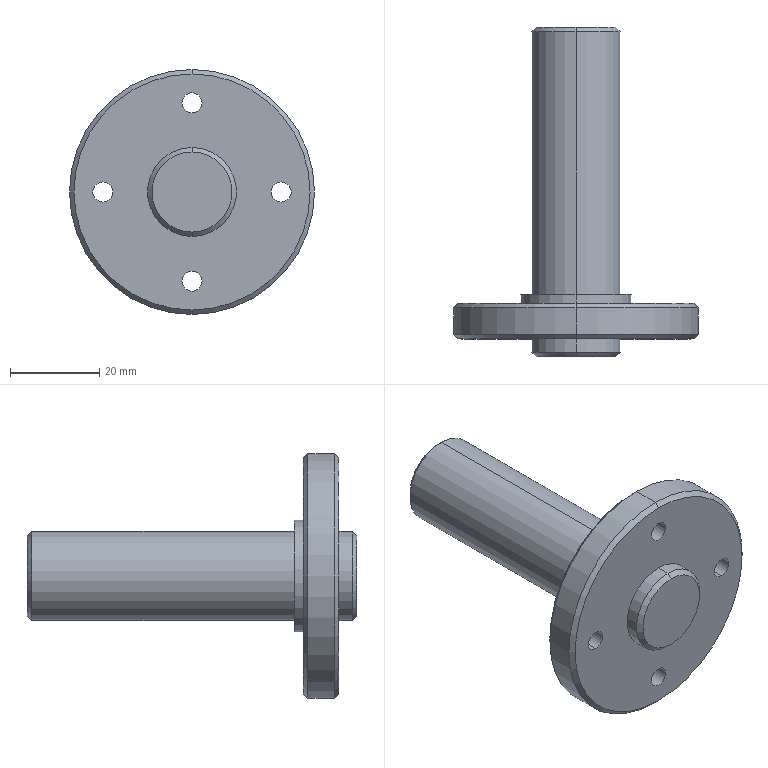Part | NX | features 00 2 | 1 solid | 41 faces | box 55 x 74 x 55 mm | volume 38722 mm3 | cylinder 24 | plane 9 | cone 8 | commonest cylinder face diameters 4.5 x8 8 x8 20 x4 25 x2 55 x2
STEP:
#1=CARTESIAN_POINT('',(0.,119.,-258.129));
#2=VERTEX_POINT('',#1);
#3=CARTESIAN_POINT('',(0.,119.,-278.129));
#4=VERTEX_POINT('',#3);
#5=CARTESIAN_POINT('',(0.,119.,-268.129));
#6=DIRECTION('',(0.,1.,0.));
#7=DIRECTION('',(0.,0.,1.));
#8=AXIS2_PLACEMENT_3D('',#5,#6,#7);
#9=CIRCLE('',#8,10.);
#10=EDGE_CURVE('',#2,#4,#9,.T.);
#11=ORIENTED_EDGE('',*,*,#10,.F.);
#12=CARTESIAN_POINT('',(0.,60.,-258.129));
#13=VERTEX_POINT('',#12);
#14=CARTESIAN_POINT('',(0.,60.,-258.129));
#15=DIRECTION('',(0.,1.,0.));
#16=VECTOR('',#15,1000.);
#17=LINE('',#14,#16);
#18=EDGE_CURVE('',#13,#2,#17,.T.);
#19=ORIENTED_EDGE('',*,*,#18,.F.);
#20=CARTESIAN_POINT('',(0.,60.,-278.129));
#21=VERTEX_POINT('',#20);
#22=CARTESIAN_POINT('',(0.,60.,-268.129));
#23=DIRECTION('',(0.,-1.,0.));
#24=DIRECTION('',(0.,0.,-1.));
#25=AXIS2_PLACEMENT_3D('',#22,#23,#24);
#26=CIRCLE('',#25,10.);
#27=EDGE_CURVE('',#21,#13,#26,.T.);
#28=ORIENTED_EDGE('',*,*,#27,.F.);
#29=CARTESIAN_POINT('',(0.,60.,-278.129));
#30=DIRECTION('',(0.,1.,0.));
#31=VECTOR('',#30,1000.);
#32=LINE('',#29,#31);
#33=EDGE_CURVE('',#4,#21,#32,.F.);
#34=ORIENTED_EDGE('',*,*,#33,.F.);
#35=EDGE_LOOP('',(#11,#19,#28,#34));
#36=FACE_BOUND('',#35,.T.);
#37=CARTESIAN_POINT('',(0.,50.,-268.129));
#38=DIRECTION('',(0.,-1.,0.));
#39=DIRECTION('',(0.,0.,1.));
#40=AXIS2_PLACEMENT_3D('',#37,#38,#39);
#41=CYLINDRICAL_SURFACE('',#40,10.);
#42=ADVANCED_FACE('',(#36),#41,.T.);
#43=CARTESIAN_POINT('',(0.,120.,-259.129));
#44=VERTEX_POINT('',#43);
#45=CARTESIAN_POINT('',(0.,120.,-277.129));
#46=VERTEX_POINT('',#45);
#47=CARTESIAN_POINT('',(0.,120.,-268.129));
#48=DIRECTION('',(0.,1.,0.));
#49=DIRECTION('',(0.,0.,1.));
#50=AXIS2_PLACEMENT_3D('',#47,#48,#49);
#51=CIRCLE('',#50,9.);
#52=EDGE_CURVE('',#44,#46,#51,.T.);
#53=ORIENTED_EDGE('',*,*,#52,.F.);
#54=CARTESIAN_POINT('',(0.,119.,-258.129));
#55=DIRECTION('',(0.,0.7071,-0.7071));
#56=VECTOR('',#55,1000.);
#57=LINE('',#54,#56);
#58=EDGE_CURVE('',#44,#2,#57,.F.);
#59=ORIENTED_EDGE('',*,*,#58,.T.);
#60=ORIENTED_EDGE('',*,*,#10,.T.);
#61=CARTESIAN_POINT('',(0.,119.,-278.129));
#62=DIRECTION('',(0.,0.7071,0.7071));
#63=VECTOR('',#62,1000.);
#64=LINE('',#61,#63);
#65=EDGE_CURVE('',#4,#46,#64,.T.);
#66=ORIENTED_EDGE('',*,*,#65,.T.);
#67=EDGE_LOOP('',(#53,#59,#60,#66));
#68=FACE_BOUND('',#67,.T.);
#69=CARTESIAN_POINT('',(0.,120.091,-268.129));
#70=DIRECTION('',(0.,-1.,0.));
#71=DIRECTION('',(0.,0.,1.));
#72=AXIS2_PLACEMENT_3D('',#69,#70,#71);
#73=CONICAL_SURFACE('',#72,8.909,0.7854);
#74=ADVANCED_FACE('',(#68),#73,.T.);
#75=CARTESIAN_POINT('',(0.,120.,-268.129));
#76=DIRECTION('',(0.,1.,0.));
#77=DIRECTION('',(0.,0.,-1.));
#78=AXIS2_PLACEMENT_3D('',#75,#76,#77);
#79=CIRCLE('',#78,9.);
#80=EDGE_CURVE('',#46,#44,#79,.T.);
#81=ORIENTED_EDGE('',*,*,#80,.T.);
#82=ORIENTED_EDGE('',*,*,#52,.T.);
#83=EDGE_LOOP('',(#81,#82));
#84=FACE_BOUND('',#83,.T.);
#85=CARTESIAN_POINT('',(-10.,120.,-268.129));
#86=DIRECTION('',(0.,1.,0.));
#87=DIRECTION('',(0.,0.,-1.));
#88=AXIS2_PLACEMENT_3D('',#85,#86,#87);
#89=PLANE('',#88);
#90=ADVANCED_FACE('',(#84),#89,.T.);
#91=ORIENTED_EDGE('',*,*,#65,.F.);
#92=CARTESIAN_POINT('',(0.,119.,-268.129));
#93=DIRECTION('',(0.,1.,0.));
#94=DIRECTION('',(0.,0.,-1.));
#95=AXIS2_PLACEMENT_3D('',#92,#93,#94);
#96=CIRCLE('',#95,10.);
#97=EDGE_CURVE('',#4,#2,#96,.T.);
#98=ORIENTED_EDGE('',*,*,#97,.T.);
#99=ORIENTED_EDGE('',*,*,#58,.F.);
#100=ORIENTED_EDGE('',*,*,#80,.F.);
#101=EDGE_LOOP('',(#91,#98,#99,#100));
#102=FACE_BOUND('',#101,.T.);
#103=CARTESIAN_POINT('',(0.,120.091,-268.129));
#104=DIRECTION('',(0.,-1.,0.));
#105=DIRECTION('',(0.,0.,1.));
#106=AXIS2_PLACEMENT_3D('',#103,#104,#105);
#107=CONICAL_SURFACE('',#106,8.909,0.7854);
#108=ADVANCED_FACE('',(#102),#107,.T.);
#109=ORIENTED_EDGE('',*,*,#33,.T.);
#110=CARTESIAN_POINT('',(0.,60.,-268.129));
#111=DIRECTION('',(0.,-1.,0.));
#112=DIRECTION('',(0.,0.,1.));
#113=AXIS2_PLACEMENT_3D('',#110,#111,#112);
#114=CIRCLE('',#113,10.);
#115=EDGE_CURVE('',#13,#21,#114,.T.);
#116=ORIENTED_EDGE('',*,*,#115,.F.);
#117=ORIENTED_EDGE('',*,*,#18,.T.);
#118=ORIENTED_EDGE('',*,*,#97,.F.);
#119=EDGE_LOOP('',(#109,#116,#117,#118));
#120=FACE_BOUND('',#119,.T.);
#121=CARTESIAN_POINT('',(0.,50.,-268.129));
#122=DIRECTION('',(0.,-1.,0.));
#123=DIRECTION('',(0.,0.,1.));
#124=AXIS2_PLACEMENT_3D('',#121,#122,#123);
#125=CYLINDRICAL_SURFACE('',#124,10.);
#126=ADVANCED_FACE('',(#120),#125,.T.);
#127=CARTESIAN_POINT('',(0.,60.,-255.629));
#128=VERTEX_POINT('',#127);
#129=CARTESIAN_POINT('',(0.,60.,-280.629));
#130=VERTEX_POINT('',#129);
#131=CARTESIAN_POINT('',(0.,60.,-268.129));
#132=DIRECTION('',(0.,1.,0.));
#133=DIRECTION('',(0.,0.,1.));
#134=AXIS2_PLACEMENT_3D('',#131,#132,#133);
#135=CIRCLE('',#134,12.5);
#136=EDGE_CURVE('',#128,#130,#135,.T.);
#137=ORIENTED_EDGE('',*,*,#136,.F.);
#138=CARTESIAN_POINT('',(0.,58.,-255.629));
#139=VERTEX_POINT('',#138);
#140=CARTESIAN_POINT('',(0.,58.,-255.629));
#141=DIRECTION('',(0.,1.,0.));
#142=VECTOR('',#141,1000.);
#143=LINE('',#140,#142);
#144=EDGE_CURVE('',#128,#139,#143,.F.);
#145=ORIENTED_EDGE('',*,*,#144,.T.);
#146=CARTESIAN_POINT('',(0.,58.,-280.629));
#147=VERTEX_POINT('',#146);
#148=CARTESIAN_POINT('',(0.,58.,-268.129));
#149=DIRECTION('',(0.,-1.,0.));
#150=DIRECTION('',(0.,0.,-1.));
#151=AXIS2_PLACEMENT_3D('',#148,#149,#150);
#152=CIRCLE('',#151,12.5);
#153=EDGE_CURVE('',#147,#139,#152,.T.);
#154=ORIENTED_EDGE('',*,*,#153,.F.);
#155=CARTESIAN_POINT('',(0.,58.,-280.629));
#156=DIRECTION('',(0.,1.,0.));
#157=VECTOR('',#156,1000.);
#158=LINE('',#155,#157);
#159=EDGE_CURVE('',#147,#130,#158,.T.);
#160=ORIENTED_EDGE('',*,*,#159,.T.);
#161=EDGE_LOOP('',(#137,#145,#154,#160));
#162=FACE_BOUND('',#161,.T.);
#163=CARTESIAN_POINT('',(0.,50.,-268.129));
#164=DIRECTION('',(0.,-1.,0.));
#165=DIRECTION('',(0.,0.,1.));
#166=AXIS2_PLACEMENT_3D('',#163,#164,#165);
#167=CYLINDRICAL_SURFACE('',#166,12.5);
#168=ADVANCED_FACE('',(#162),#167,.T.);
#169=ORIENTED_EDGE('',*,*,#27,.T.);
#170=ORIENTED_EDGE('',*,*,#115,.T.);
#171=EDGE_LOOP('',(#169,#170));
#172=FACE_BOUND('',#171,.T.);
#173=ORIENTED_EDGE('',*,*,#136,.T.);
#174=CARTESIAN_POINT('',(0.,60.,-268.129));
#175=DIRECTION('',(0.,1.,0.));
#176=DIRECTION('',(0.,0.,-1.));
#177=AXIS2_PLACEMENT_3D('',#174,#175,#176);
#178=CIRCLE('',#177,12.5);
#179=EDGE_CURVE('',#130,#128,#178,.T.);
#180=ORIENTED_EDGE('',*,*,#179,.T.);
#181=EDGE_LOOP('',(#173,#180));
#182=FACE_BOUND('',#181,.T.);
#183=CARTESIAN_POINT('',(-12.5,60.,-268.129));
#184=DIRECTION('',(0.,1.,0.));
#185=DIRECTION('',(0.,0.,-1.));
#186=AXIS2_PLACEMENT_3D('',#183,#184,#185);
#187=PLANE('',#186);
#188=ADVANCED_FACE('',(#172,#182),#187,.T.);
#189=ORIENTED_EDGE('',*,*,#159,.F.);
#190=CARTESIAN_POINT('',(0.,58.,-268.129));
#191=DIRECTION('',(0.,-1.,0.));
#192=DIRECTION('',(0.,0.,1.));
#193=AXIS2_PLACEMENT_3D('',#190,#191,#192);
#194=CIRCLE('',#193,12.5);
#195=EDGE_CURVE('',#139,#147,#194,.T.);
#196=ORIENTED_EDGE('',*,*,#195,.F.);
#197=ORIENTED_EDGE('',*,*,#144,.F.);
#198=ORIENTED_EDGE('',*,*,#179,.F.);
#199=EDGE_LOOP('',(#189,#196,#197,#198));
#200=FACE_BOUND('',#199,.T.);
#201=CARTESIAN_POINT('',(0.,50.,-268.129));
#202=DIRECTION('',(0.,-1.,0.));
#203=DIRECTION('',(0.,0.,1.));
#204=AXIS2_PLACEMENT_3D('',#201,#202,#203);
#205=CYLINDRICAL_SURFACE('',#204,12.5);
#206=ADVANCED_FACE('',(#200),#205,.T.);
#207=CARTESIAN_POINT('',(-20.,53.4,-265.879));
#208=VERTEX_POINT('',#207);
#209=CARTESIAN_POINT('',(-20.,50.,-265.879));
#210=VERTEX_POINT('',#209);
#211=CARTESIAN_POINT('',(-20.,53.4,-265.879));
#212=DIRECTION('',(0.,-1.,0.));
#213=VECTOR('',#212,1000.);
#214=LINE('',#211,#213);
#215=EDGE_CURVE('',#208,#210,#214,.T.);
#216=ORIENTED_EDGE('',*,*,#215,.F.);
#217=CARTESIAN_POINT('',(-20.,53.4,-270.379));
#218=VERTEX_POINT('',#217);
#219=CARTESIAN_POINT('',(-20.,53.4,-268.129));
#220=DIRECTION('',(0.,-1.,0.));
#221=DIRECTION('',(0.,0.,-1.));
#222=AXIS2_PLACEMENT_3D('',#219,#220,#221);
#223=CIRCLE('',#222,2.25);
#224=EDGE_CURVE('',#218,#208,#223,.T.);
#225=ORIENTED_EDGE('',*,*,#224,.F.);
#226=CARTESIAN_POINT('',(-20.,50.,-270.379));
#227=VERTEX_POINT('',#226);
#228=CARTESIAN_POINT('',(-20.,53.4,-270.379));
#229=DIRECTION('',(0.,-1.,0.));
#230=VECTOR('',#229,1000.);
#231=LINE('',#228,#230);
#232=EDGE_CURVE('',#227,#218,#231,.F.);
#233=ORIENTED_EDGE('',*,*,#232,.F.);
#234=CARTESIAN_POINT('',(-20.,50.,-268.129));
#235=DIRECTION('',(0.,1.,0.));
#236=DIRECTION('',(0.,0.,1.));
#237=AXIS2_PLACEMENT_3D('',#234,#235,#236);
#238=CIRCLE('',#237,2.25);
#239=EDGE_CURVE('',#210,#227,#238,.T.);
#240=ORIENTED_EDGE('',*,*,#239,.F.);
#241=EDGE_LOOP('',(#216,#225,#233,#240));
#242=FACE_BOUND('',#241,.T.);
#243=CARTESIAN_POINT('',(-20.,58.,-268.129));
#244=DIRECTION('',(0.,1.,0.));
#245=DIRECTION('',(0.,0.,-1.));
#246=AXIS2_PLACEMENT_3D('',#243,#244,#245);
#247=CYLINDRICAL_SURFACE('',#246,2.25);
#248=ADVANCED_FACE('',(#242),#247,.F.);
#249=CARTESIAN_POINT('',(-20.,50.,-268.129));
#250=DIRECTION('',(0.,1.,0.));
#251=DIRECTION('',(0.,0.,-1.));
#252=AXIS2_PLACEMENT_3D('',#249,#250,#251);
#253=CIRCLE('',#252,2.25);
#254=EDGE_CURVE('',#227,#210,#253,.T.);
#255=ORIENTED_EDGE('',*,*,#254,.F.);
#256=ORIENTED_EDGE('',*,*,#232,.T.);
#257=CARTESIAN_POINT('',(-20.,53.4,-268.129));
#258=DIRECTION('',(0.,-1.,0.));
#259=DIRECTION('',(0.,0.,1.));
#260=AXIS2_PLACEMENT_3D('',#257,#258,#259);
#261=CIRCLE('',#260,2.25);
#262=EDGE_CURVE('',#208,#218,#261,.T.);
#263=ORIENTED_EDGE('',*,*,#262,.F.);
#264=ORIENTED_EDGE('',*,*,#215,.T.);
#265=EDGE_LOOP('',(#255,#256,#263,#264));
#266=FACE_BOUND('',#265,.T.);
#267=CARTESIAN_POINT('',(-20.,58.,-268.129));
#268=DIRECTION('',(0.,1.,0.));
#269=DIRECTION('',(0.,0.,-1.));
#270=AXIS2_PLACEMENT_3D('',#267,#268,#269);
#271=CYLINDRICAL_SURFACE('',#270,2.25);
#272=ADVANCED_FACE('',(#266),#271,.F.);
#273=ORIENTED_EDGE('',*,*,#224,.T.);
#274=ORIENTED_EDGE('',*,*,#262,.T.);
#275=EDGE_LOOP('',(#273,#274));
#276=FACE_BOUND('',#275,.T.);
#277=CARTESIAN_POINT('',(-20.,53.4,-264.129));
#278=VERTEX_POINT('',#277);
#279=CARTESIAN_POINT('',(-20.,53.4,-272.129));
#280=VERTEX_POINT('',#279);
#281=CARTESIAN_POINT('',(-20.,53.4,-268.129));
#282=DIRECTION('',(0.,1.,0.));
#283=DIRECTION('',(0.,0.,1.));
#284=AXIS2_PLACEMENT_3D('',#281,#282,#283);
#285=CIRCLE('',#284,4.);
#286=EDGE_CURVE('',#278,#280,#285,.T.);
#287=ORIENTED_EDGE('',*,*,#286,.T.);
#288=CARTESIAN_POINT('',(-20.,53.4,-268.129));
#289=DIRECTION('',(0.,1.,0.));
#290=DIRECTION('',(0.,0.,-1.));
#291=AXIS2_PLACEMENT_3D('',#288,#289,#290);
#292=CIRCLE('',#291,4.);
#293=EDGE_CURVE('',#280,#278,#292,.T.);
#294=ORIENTED_EDGE('',*,*,#293,.T.);
#295=EDGE_LOOP('',(#287,#294));
#296=FACE_BOUND('',#295,.T.);
#297=CARTESIAN_POINT('',(-22.25,53.4,-268.129));
#298=DIRECTION('',(0.,-1.,0.));
#299=DIRECTION('',(0.,0.,1.));
#300=AXIS2_PLACEMENT_3D('',#297,#298,#299);
#301=PLANE('',#300);
#302=ADVANCED_FACE('',(#276,#296),#301,.F.);
#303=CARTESIAN_POINT('',(-20.,58.,-264.129));
#304=VERTEX_POINT('',#303);
#305=CARTESIAN_POINT('',(-20.,58.,-264.129));
#306=DIRECTION('',(0.,-1.,0.));
#307=VECTOR('',#306,1000.);
#308=LINE('',#305,#307);
#309=EDGE_CURVE('',#304,#278,#308,.T.);
#310=ORIENTED_EDGE('',*,*,#309,.F.);
#311=CARTESIAN_POINT('',(-20.,58.,-272.129));
#312=VERTEX_POINT('',#311);
#313=CARTESIAN_POINT('',(-20.,58.,-268.129));
#314=DIRECTION('',(0.,-1.,0.));
#315=DIRECTION('',(0.,0.,-1.));
#316=AXIS2_PLACEMENT_3D('',#313,#314,#315);
#317=CIRCLE('',#316,4.);
#318=EDGE_CURVE('',#312,#304,#317,.T.);
#319=ORIENTED_EDGE('',*,*,#318,.F.);
#320=CARTESIAN_POINT('',(-20.,58.,-272.129));
#321=DIRECTION('',(0.,-1.,0.));
#322=VECTOR('',#321,1000.);
#323=LINE('',#320,#322);
#324=EDGE_CURVE('',#280,#312,#323,.F.);
#325=ORIENTED_EDGE('',*,*,#324,.F.);
#326=ORIENTED_EDGE('',*,*,#286,.F.);
#327=EDGE_LOOP('',(#310,#319,#325,#326));
#328=FACE_BOUND('',#327,.T.);
#329=CARTESIAN_POINT('',(-20.,58.,-268.129));
#330=DIRECTION('',(0.,1.,0.));
#331=DIRECTION('',(0.,0.,-1.));
#332=AXIS2_PLACEMENT_3D('',#329,#330,#331);
#333=CYLINDRICAL_SURFACE('',#332,4.);
#334=ADVANCED_FACE('',(#328),#333,.F.);
#335=ORIENTED_EDGE('',*,*,#293,.F.);
#336=ORIENTED_EDGE('',*,*,#324,.T.);
#337=CARTESIAN_POINT('',(-20.,58.,-268.129));
#338=DIRECTION('',(0.,-1.,0.));
#339=DIRECTION('',(0.,0.,1.));
#340=AXIS2_PLACEMENT_3D('',#337,#338,#339);
#341=CIRCLE('',#340,4.);
#342=EDGE_CURVE('',#304,#312,#341,.T.);
#343=ORIENTED_EDGE('',*,*,#342,.F.);
#344=ORIENTED_EDGE('',*,*,#309,.T.);
#345=EDGE_LOOP('',(#335,#336,#343,#344));
#346=FACE_BOUND('',#345,.T.);
#347=CARTESIAN_POINT('',(-20.,58.,-268.129));
#348=DIRECTION('',(0.,1.,0.));
#349=DIRECTION('',(0.,0.,-1.));
#350=AXIS2_PLACEMENT_3D('',#347,#348,#349);
#351=CYLINDRICAL_SURFACE('',#350,4.);
#352=ADVANCED_FACE('',(#346),#351,.F.);
#353=CARTESIAN_POINT('',(-2.25,50.,-288.129));
#354=VERTEX_POINT('',#353);
#355=CARTESIAN_POINT('',(-2.25,53.4,-288.129));
#356=VERTEX_POINT('',#355);
#357=CARTESIAN_POINT('',(-2.25,53.4,-288.129));
#358=DIRECTION('',(0.,-1.,0.));
#359=VECTOR('',#358,1000.);
#360=LINE('',#357,#359);
#361=EDGE_CURVE('',#354,#356,#360,.F.);
#362=ORIENTED_EDGE('',*,*,#361,.T.);
#363=CARTESIAN_POINT('',(2.25,53.4,-288.129));
#364=VERTEX_POINT('',#363);
#365=CARTESIAN_POINT('',(0.,53.4,-288.129));
#366=DIRECTION('',(0.,-1.,0.));
#367=DIRECTION('',(1.,0.,0.));
#368=AXIS2_PLACEMENT_3D('',#365,#366,#367);
#369=CIRCLE('',#368,2.25);
#370=EDGE_CURVE('',#364,#356,#369,.T.);
#371=ORIENTED_EDGE('',*,*,#370,.F.);
#372=CARTESIAN_POINT('',(2.25,50.,-288.129));
#373=VERTEX_POINT('',#372);
#374=CARTESIAN_POINT('',(2.25,53.4,-288.129));
#375=DIRECTION('',(0.,-1.,0.));
#376=VECTOR('',#375,1000.);
#377=LINE('',#374,#376);
#378=EDGE_CURVE('',#364,#373,#377,.T.);
#379=ORIENTED_EDGE('',*,*,#378,.T.);
#380=CARTESIAN_POINT('',(0.,50.,-288.129));
#381=DIRECTION('',(0.,1.,0.));
#382=DIRECTION('',(-1.,0.,0.));
#383=AXIS2_PLACEMENT_3D('',#380,#381,#382);
#384=CIRCLE('',#383,2.25);
#385=EDGE_CURVE('',#354,#373,#384,.T.);
#386=ORIENTED_EDGE('',*,*,#385,.F.);
#387=EDGE_LOOP('',(#362,#371,#379,#386));
#388=FACE_BOUND('',#387,.T.);
#389=CARTESIAN_POINT('',(0.,58.,-288.129));
#390=DIRECTION('',(0.,1.,0.));
#391=DIRECTION('',(1.,0.,0.));
#392=AXIS2_PLACEMENT_3D('',#389,#390,#391);
#393=CYLINDRICAL_SURFACE('',#392,2.25);
#394=ADVANCED_FACE('',(#388),#393,.F.);
#395=CARTESIAN_POINT('',(0.,50.,-288.129));
#396=DIRECTION('',(0.,1.,0.));
#397=DIRECTION('',(1.,0.,0.));
#398=AXIS2_PLACEMENT_3D('',#395,#396,#397);
#399=CIRCLE('',#398,2.25);
#400=EDGE_CURVE('',#373,#354,#399,.T.);
#401=ORIENTED_EDGE('',*,*,#400,.F.);
#402=ORIENTED_EDGE('',*,*,#378,.F.);
#403=CARTESIAN_POINT('',(0.,53.4,-288.129));
#404=DIRECTION('',(0.,-1.,0.));
#405=DIRECTION('',(-1.,0.,0.));
#406=AXIS2_PLACEMENT_3D('',#403,#404,#405);
#407=CIRCLE('',#406,2.25);
#408=EDGE_CURVE('',#356,#364,#407,.T.);
#409=ORIENTED_EDGE('',*,*,#408,.F.);
#410=ORIENTED_EDGE('',*,*,#361,.F.);
#411=EDGE_LOOP('',(#401,#402,#409,#410));
#412=FACE_BOUND('',#411,.T.);
#413=CARTESIAN_POINT('',(0.,58.,-288.129));
#414=DIRECTION('',(0.,1.,0.));
#415=DIRECTION('',(1.,0.,0.));
#416=AXIS2_PLACEMENT_3D('',#413,#414,#415);
#417=CYLINDRICAL_SURFACE('',#416,2.25);
#418=ADVANCED_FACE('',(#412),#417,.F.);
#419=ORIENTED_EDGE('',*,*,#370,.T.);
#420=ORIENTED_EDGE('',*,*,#408,.T.);
#421=EDGE_LOOP('',(#419,#420));
#422=FACE_BOUND('',#421,.T.);
#423=CARTESIAN_POINT('',(-4.,53.4,-288.129));
#424=VERTEX_POINT('',#423);
#425=CARTESIAN_POINT('',(4.,53.4,-288.129));
#426=VERTEX_POINT('',#425);
#427=CARTESIAN_POINT('',(0.,53.4,-288.129));
#428=DIRECTION('',(0.,1.,0.));
#429=DIRECTION('',(-1.,0.,0.));
#430=AXIS2_PLACEMENT_3D('',#427,#428,#429);
#431=CIRCLE('',#430,4.);
#432=EDGE_CURVE('',#424,#426,#431,.T.);
#433=ORIENTED_EDGE('',*,*,#432,.T.);
#434=CARTESIAN_POINT('',(0.,53.4,-288.129));
#435=DIRECTION('',(0.,1.,0.));
#436=DIRECTION('',(1.,0.,0.));
#437=AXIS2_PLACEMENT_3D('',#434,#435,#436);
#438=CIRCLE('',#437,4.);
#439=EDGE_CURVE('',#426,#424,#438,.T.);
#440=ORIENTED_EDGE('',*,*,#439,.T.);
#441=EDGE_LOOP('',(#433,#440));
#442=FACE_BOUND('',#441,.T.);
#443=CARTESIAN_POINT('',(0.,53.4,-290.379));
#444=DIRECTION('',(0.,-1.,0.));
#445=DIRECTION('',(-1.,0.,0.));
#446=AXIS2_PLACEMENT_3D('',#443,#444,#445);
#447=PLANE('',#446);
#448=ADVANCED_FACE('',(#422,#442),#447,.F.);
#449=CARTESIAN_POINT('',(-4.,58.,-288.129));
#450=VERTEX_POINT('',#449);
#451=CARTESIAN_POINT('',(-4.,58.,-288.129));
#452=DIRECTION('',(0.,-1.,0.));
#453=VECTOR('',#452,1000.);
#454=LINE('',#451,#453);
#455=EDGE_CURVE('',#450,#424,#454,.T.);
#456=ORIENTED_EDGE('',*,*,#455,.F.);
#457=CARTESIAN_POINT('',(4.,58.,-288.129));
#458=VERTEX_POINT('',#457);
#459=CARTESIAN_POINT('',(0.,58.,-288.129));
#460=DIRECTION('',(0.,-1.,0.));
#461=DIRECTION('',(1.,0.,0.));
#462=AXIS2_PLACEMENT_3D('',#459,#460,#461);
#463=CIRCLE('',#462,4.);
#464=EDGE_CURVE('',#458,#450,#463,.T.);
#465=ORIENTED_EDGE('',*,*,#464,.F.);
#466=CARTESIAN_POINT('',(4.,58.,-288.129));
#467=DIRECTION('',(0.,-1.,0.));
#468=VECTOR('',#467,1000.);
#469=LINE('',#466,#468);
#470=EDGE_CURVE('',#426,#458,#469,.F.);
#471=ORIENTED_EDGE('',*,*,#470,.F.);
#472=ORIENTED_EDGE('',*,*,#432,.F.);
#473=EDGE_LOOP('',(#456,#465,#471,#472));
#474=FACE_BOUND('',#473,.T.);
#475=CARTESIAN_POINT('',(0.,58.,-288.129));
#476=DIRECTION('',(0.,1.,0.));
#477=DIRECTION('',(1.,0.,0.));
#478=AXIS2_PLACEMENT_3D('',#475,#476,#477);
#479=CYLINDRICAL_SURFACE('',#478,4.);
#480=ADVANCED_FACE('',(#474),#479,.F.);
#481=ORIENTED_EDGE('',*,*,#439,.F.);
#482=ORIENTED_EDGE('',*,*,#470,.T.);
#483=CARTESIAN_POINT('',(0.,58.,-288.129));
#484=DIRECTION('',(0.,-1.,0.));
#485=DIRECTION('',(-1.,0.,0.));
#486=AXIS2_PLACEMENT_3D('',#483,#484,#485);
#487=CIRCLE('',#486,4.);
#488=EDGE_CURVE('',#450,#458,#487,.T.);
#489=ORIENTED_EDGE('',*,*,#488,.F.);
#490=ORIENTED_EDGE('',*,*,#455,.T.);
#491=EDGE_LOOP('',(#481,#482,#489,#490));
#492=FACE_BOUND('',#491,.T.);
#493=CARTESIAN_POINT('',(0.,58.,-288.129));
#494=DIRECTION('',(0.,1.,0.));
#495=DIRECTION('',(1.,0.,0.));
#496=AXIS2_PLACEMENT_3D('',#493,#494,#495);
#497=CYLINDRICAL_SURFACE('',#496,4.);
#498=ADVANCED_FACE('',(#492),#497,.F.);
#499=CARTESIAN_POINT('',(20.,53.4,-270.379));
#500=VERTEX_POINT('',#499);
#501=CARTESIAN_POINT('',(20.,50.,-270.379));
#502=VERTEX_POINT('',#501);
#503=CARTESIAN_POINT('',(20.,53.4,-270.379));
#504=DIRECTION('',(0.,-1.,0.));
#505=VECTOR('',#504,1000.);
#506=LINE('',#503,#505);
#507=EDGE_CURVE('',#500,#502,#506,.T.);
#508=ORIENTED_EDGE('',*,*,#507,.F.);
#509=CARTESIAN_POINT('',(20.,53.4,-265.879));
#510=VERTEX_POINT('',#509);
#511=CARTESIAN_POINT('',(20.,53.4,-268.129));
#512=DIRECTION('',(0.,-1.,0.));
#513=DIRECTION('',(0.,0.,1.));
#514=AXIS2_PLACEMENT_3D('',#511,#512,#513);
#515=CIRCLE('',#514,2.25);
#516=EDGE_CURVE('',#510,#500,#515,.T.);
#517=ORIENTED_EDGE('',*,*,#516,.F.);
#518=CARTESIAN_POINT('',(20.,50.,-265.879));
#519=VERTEX_POINT('',#518);
#520=CARTESIAN_POINT('',(20.,53.4,-265.879));
#521=DIRECTION('',(0.,-1.,0.));
#522=VECTOR('',#521,1000.);
#523=LINE('',#520,#522);
#524=EDGE_CURVE('',#519,#510,#523,.F.);
#525=ORIENTED_EDGE('',*,*,#524,.F.);
#526=CARTESIAN_POINT('',(20.,50.,-268.129));
#527=DIRECTION('',(0.,1.,0.));
#528=DIRECTION('',(0.,0.,-1.));
#529=AXIS2_PLACEMENT_3D('',#526,#527,#528);
#530=CIRCLE('',#529,2.25);
#531=EDGE_CURVE('',#502,#519,#530,.T.);
#532=ORIENTED_EDGE('',*,*,#531,.F.);
#533=EDGE_LOOP('',(#508,#517,#525,#532));
#534=FACE_BOUND('',#533,.T.);
#535=CARTESIAN_POINT('',(20.,58.,-268.129));
#536=DIRECTION('',(0.,1.,0.));
#537=DIRECTION('',(0.,0.,1.));
#538=AXIS2_PLACEMENT_3D('',#535,#536,#537);
#539=CYLINDRICAL_SURFACE('',#538,2.25);
#540=ADVANCED_FACE('',(#534),#539,.F.);
#541=CARTESIAN_POINT('',(20.,50.,-268.129));
#542=DIRECTION('',(0.,1.,0.));
#543=DIRECTION('',(0.,0.,1.));
#544=AXIS2_PLACEMENT_3D('',#541,#542,#543);
#545=CIRCLE('',#544,2.25);
#546=EDGE_CURVE('',#519,#502,#545,.T.);
#547=ORIENTED_EDGE('',*,*,#546,.F.);
#548=ORIENTED_EDGE('',*,*,#524,.T.);
#549=CARTESIAN_POINT('',(20.,53.4,-268.129));
#550=DIRECTION('',(0.,-1.,0.));
#551=DIRECTION('',(0.,0.,-1.));
#552=AXIS2_PLACEMENT_3D('',#549,#550,#551);
#553=CIRCLE('',#552,2.25);
#554=EDGE_CURVE('',#500,#510,#553,.T.);
#555=ORIENTED_EDGE('',*,*,#554,.F.);
#556=ORIENTED_EDGE('',*,*,#507,.T.);
#557=EDGE_LOOP('',(#547,#548,#555,#556));
#558=FACE_BOUND('',#557,.T.);
#559=CARTESIAN_POINT('',(20.,58.,-268.129));
#560=DIRECTION('',(0.,1.,0.));
#561=DIRECTION('',(0.,0.,1.));
#562=AXIS2_PLACEMENT_3D('',#559,#560,#561);
#563=CYLINDRICAL_SURFACE('',#562,2.25);
#564=ADVANCED_FACE('',(#558),#563,.F.);
#565=ORIENTED_EDGE('',*,*,#516,.T.);
#566=ORIENTED_EDGE('',*,*,#554,.T.);
#567=EDGE_LOOP('',(#565,#566));
#568=FACE_BOUND('',#567,.T.);
#569=CARTESIAN_POINT('',(20.,53.4,-272.129));
#570=VERTEX_POINT('',#569);
#571=CARTESIAN_POINT('',(20.,53.4,-264.129));
#572=VERTEX_POINT('',#571);
#573=CARTESIAN_POINT('',(20.,53.4,-268.129));
#574=DIRECTION('',(0.,1.,0.));
#575=DIRECTION('',(0.,0.,-1.));
#576=AXIS2_PLACEMENT_3D('',#573,#574,#575);
#577=CIRCLE('',#576,4.);
#578=EDGE_CURVE('',#570,#572,#577,.T.);
#579=ORIENTED_EDGE('',*,*,#578,.T.);
#580=CARTESIAN_POINT('',(20.,53.4,-268.129));
#581=DIRECTION('',(0.,1.,0.));
#582=DIRECTION('',(0.,0.,1.));
#583=AXIS2_PLACEMENT_3D('',#580,#581,#582);
#584=CIRCLE('',#583,4.);
#585=EDGE_CURVE('',#572,#570,#584,.T.);
#586=ORIENTED_EDGE('',*,*,#585,.T.);
#587=EDGE_LOOP('',(#579,#586));
#588=FACE_BOUND('',#587,.T.);
#589=CARTESIAN_POINT('',(22.25,53.4,-268.129));
#590=DIRECTION('',(0.,-1.,0.));
#591=DIRECTION('',(0.,0.,-1.));
#592=AXIS2_PLACEMENT_3D('',#589,#590,#591);
#593=PLANE('',#592);
#594=ADVANCED_FACE('',(#568,#588),#593,.F.);
#595=CARTESIAN_POINT('',(20.,58.,-272.129));
#596=VERTEX_POINT('',#595);
#597=CARTESIAN_POINT('',(20.,58.,-272.129));
#598=DIRECTION('',(0.,-1.,0.));
#599=VECTOR('',#598,1000.);
#600=LINE('',#597,#599);
#601=EDGE_CURVE('',#570,#596,#600,.F.);
#602=ORIENTED_EDGE('',*,*,#601,.T.);
#603=CARTESIAN_POINT('',(20.,58.,-264.129));
#604=VERTEX_POINT('',#603);
#605=CARTESIAN_POINT('',(20.,58.,-268.129));
#606=DIRECTION('',(0.,-1.,0.));
#607=DIRECTION('',(0.,0.,1.));
#608=AXIS2_PLACEMENT_3D('',#605,#606,#607);
#609=CIRCLE('',#608,4.);
#610=EDGE_CURVE('',#604,#596,#609,.T.);
#611=ORIENTED_EDGE('',*,*,#610,.F.);
#612=CARTESIAN_POINT('',(20.,58.,-264.129));
#613=DIRECTION('',(0.,-1.,0.));
#614=VECTOR('',#613,1000.);
#615=LINE('',#612,#614);
#616=EDGE_CURVE('',#604,#572,#615,.T.);
#617=ORIENTED_EDGE('',*,*,#616,.T.);
#618=ORIENTED_EDGE('',*,*,#578,.F.);
#619=EDGE_LOOP('',(#602,#611,#617,#618));
#620=FACE_BOUND('',#619,.T.);
#621=CARTESIAN_POINT('',(20.,58.,-268.129));
#622=DIRECTION('',(0.,1.,0.));
#623=DIRECTION('',(0.,0.,1.));
#624=AXIS2_PLACEMENT_3D('',#621,#622,#623);
#625=CYLINDRICAL_SURFACE('',#624,4.);
#626=ADVANCED_FACE('',(#620),#625,.F.);
#627=ORIENTED_EDGE('',*,*,#585,.F.);
#628=ORIENTED_EDGE('',*,*,#616,.F.);
#629=CARTESIAN_POINT('',(20.,58.,-268.129));
#630=DIRECTION('',(0.,-1.,0.));
#631=DIRECTION('',(0.,0.,-1.));
#632=AXIS2_PLACEMENT_3D('',#629,#630,#631);
#633=CIRCLE('',#632,4.);
#634=EDGE_CURVE('',#596,#604,#633,.T.);
#635=ORIENTED_EDGE('',*,*,#634,.F.);
#636=ORIENTED_EDGE('',*,*,#601,.F.);
#637=EDGE_LOOP('',(#627,#628,#635,#636));
#638=FACE_BOUND('',#637,.T.);
#639=CARTESIAN_POINT('',(20.,58.,-268.129));
#640=DIRECTION('',(0.,1.,0.));
#641=DIRECTION('',(0.,0.,1.));
#642=AXIS2_PLACEMENT_3D('',#639,#640,#641);
#643=CYLINDRICAL_SURFACE('',#642,4.);
#644=ADVANCED_FACE('',(#638),#643,.F.);
#645=CARTESIAN_POINT('',(2.25,50.,-248.129));
#646=VERTEX_POINT('',#645);
#647=CARTESIAN_POINT('',(2.25,53.4,-248.129));
#648=VERTEX_POINT('',#647);
#649=CARTESIAN_POINT('',(2.25,53.4,-248.129));
#650=DIRECTION('',(0.,-1.,0.));
#651=VECTOR('',#650,1000.);
#652=LINE('',#649,#651);
#653=EDGE_CURVE('',#646,#648,#652,.F.);
#654=ORIENTED_EDGE('',*,*,#653,.T.);
#655=CARTESIAN_POINT('',(-2.25,53.4,-248.129));
#656=VERTEX_POINT('',#655);
#657=CARTESIAN_POINT('',(0.,53.4,-248.129));
#658=DIRECTION('',(0.,-1.,0.));
#659=DIRECTION('',(-1.,0.,0.));
#660=AXIS2_PLACEMENT_3D('',#657,#658,#659);
#661=CIRCLE('',#660,2.25);
#662=EDGE_CURVE('',#656,#648,#661,.T.);
#663=ORIENTED_EDGE('',*,*,#662,.F.);
#664=CARTESIAN_POINT('',(-2.25,50.,-248.129));
#665=VERTEX_POINT('',#664);
#666=CARTESIAN_POINT('',(-2.25,53.4,-248.129));
#667=DIRECTION('',(0.,-1.,0.));
#668=VECTOR('',#667,1000.);
#669=LINE('',#666,#668);
#670=EDGE_CURVE('',#656,#665,#669,.T.);
#671=ORIENTED_EDGE('',*,*,#670,.T.);
#672=CARTESIAN_POINT('',(0.,50.,-248.129));
#673=DIRECTION('',(0.,1.,0.));
#674=DIRECTION('',(1.,0.,0.));
#675=AXIS2_PLACEMENT_3D('',#672,#673,#674);
#676=CIRCLE('',#675,2.25);
#677=EDGE_CURVE('',#646,#665,#676,.T.);
#678=ORIENTED_EDGE('',*,*,#677,.F.);
#679=EDGE_LOOP('',(#654,#663,#671,#678));
#680=FACE_BOUND('',#679,.T.);
#681=CARTESIAN_POINT('',(0.,58.,-248.129));
#682=DIRECTION('',(0.,1.,0.));
#683=DIRECTION('',(-1.,0.,0.));
#684=AXIS2_PLACEMENT_3D('',#681,#682,#683);
#685=CYLINDRICAL_SURFACE('',#684,2.25);
#686=ADVANCED_FACE('',(#680),#685,.F.);
#687=CARTESIAN_POINT('',(0.,50.,-248.129));
#688=DIRECTION('',(0.,1.,0.));
#689=DIRECTION('',(-1.,0.,0.));
#690=AXIS2_PLACEMENT_3D('',#687,#688,#689);
#691=CIRCLE('',#690,2.25);
#692=EDGE_CURVE('',#665,#646,#691,.T.);
#693=ORIENTED_EDGE('',*,*,#692,.F.);
#694=ORIENTED_EDGE('',*,*,#670,.F.);
#695=CARTESIAN_POINT('',(0.,53.4,-248.129));
#696=DIRECTION('',(0.,-1.,0.));
#697=DIRECTION('',(1.,0.,0.));
#698=AXIS2_PLACEMENT_3D('',#695,#696,#697);
#699=CIRCLE('',#698,2.25);
#700=EDGE_CURVE('',#648,#656,#699,.T.);
#701=ORIENTED_EDGE('',*,*,#700,.F.);
#702=ORIENTED_EDGE('',*,*,#653,.F.);
#703=EDGE_LOOP('',(#693,#694,#701,#702));
#704=FACE_BOUND('',#703,.T.);
#705=CARTESIAN_POINT('',(0.,58.,-248.129));
#706=DIRECTION('',(0.,1.,0.));
#707=DIRECTION('',(-1.,0.,0.));
#708=AXIS2_PLACEMENT_3D('',#705,#706,#707);
#709=CYLINDRICAL_SURFACE('',#708,2.25);
#710=ADVANCED_FACE('',(#704),#709,.F.);
#711=ORIENTED_EDGE('',*,*,#662,.T.);
#712=ORIENTED_EDGE('',*,*,#700,.T.);
#713=EDGE_LOOP('',(#711,#712));
#714=FACE_BOUND('',#713,.T.);
#715=CARTESIAN_POINT('',(4.,53.4,-248.129));
#716=VERTEX_POINT('',#715);
#717=CARTESIAN_POINT('',(-4.,53.4,-248.129));
#718=VERTEX_POINT('',#717);
#719=CARTESIAN_POINT('',(0.,53.4,-248.129));
#720=DIRECTION('',(0.,1.,0.));
#721=DIRECTION('',(1.,0.,0.));
#722=AXIS2_PLACEMENT_3D('',#719,#720,#721);
#723=CIRCLE('',#722,4.);
#724=EDGE_CURVE('',#716,#718,#723,.T.);
#725=ORIENTED_EDGE('',*,*,#724,.T.);
#726=CARTESIAN_POINT('',(0.,53.4,-248.129));
#727=DIRECTION('',(0.,1.,0.));
#728=DIRECTION('',(-1.,0.,0.));
#729=AXIS2_PLACEMENT_3D('',#726,#727,#728);
#730=CIRCLE('',#729,4.);
#731=EDGE_CURVE('',#718,#716,#730,.T.);
#732=ORIENTED_EDGE('',*,*,#731,.T.);
#733=EDGE_LOOP('',(#725,#732));
#734=FACE_BOUND('',#733,.T.);
#735=CARTESIAN_POINT('',(0.,53.4,-245.879));
#736=DIRECTION('',(0.,-1.,0.));
#737=DIRECTION('',(1.,0.,0.));
#738=AXIS2_PLACEMENT_3D('',#735,#736,#737);
#739=PLANE('',#738);
#740=ADVANCED_FACE('',(#714,#734),#739,.F.);
#741=CARTESIAN_POINT('',(4.,58.,-248.129));
#742=VERTEX_POINT('',#741);
#743=CARTESIAN_POINT('',(4.,58.,-248.129));
#744=DIRECTION('',(0.,-1.,0.));
#745=VECTOR('',#744,1000.);
#746=LINE('',#743,#745);
#747=EDGE_CURVE('',#742,#716,#746,.T.);
#748=ORIENTED_EDGE('',*,*,#747,.F.);
#749=CARTESIAN_POINT('',(-4.,58.,-248.129));
#750=VERTEX_POINT('',#749);
#751=CARTESIAN_POINT('',(0.,58.,-248.129));
#752=DIRECTION('',(0.,-1.,0.));
#753=DIRECTION('',(-1.,0.,0.));
#754=AXIS2_PLACEMENT_3D('',#751,#752,#753);
#755=CIRCLE('',#754,4.);
#756=EDGE_CURVE('',#750,#742,#755,.T.);
#757=ORIENTED_EDGE('',*,*,#756,.F.);
#758=CARTESIAN_POINT('',(-4.,58.,-248.129));
#759=DIRECTION('',(0.,-1.,0.));
#760=VECTOR('',#759,1000.);
#761=LINE('',#758,#760);
#762=EDGE_CURVE('',#718,#750,#761,.F.);
#763=ORIENTED_EDGE('',*,*,#762,.F.);
#764=ORIENTED_EDGE('',*,*,#724,.F.);
#765=EDGE_LOOP('',(#748,#757,#763,#764));
#766=FACE_BOUND('',#765,.T.);
#767=CARTESIAN_POINT('',(0.,58.,-248.129));
#768=DIRECTION('',(0.,1.,0.));
#769=DIRECTION('',(-1.,0.,0.));
#770=AXIS2_PLACEMENT_3D('',#767,#768,#769);
#771=CYLINDRICAL_SURFACE('',#770,4.);
#772=ADVANCED_FACE('',(#766),#771,.F.);
#773=ORIENTED_EDGE('',*,*,#731,.F.);
#774=ORIENTED_EDGE('',*,*,#762,.T.);
#775=CARTESIAN_POINT('',(0.,58.,-248.129));
#776=DIRECTION('',(0.,-1.,0.));
#777=DIRECTION('',(1.,0.,0.));
#778=AXIS2_PLACEMENT_3D('',#775,#776,#777);
#779=CIRCLE('',#778,4.);
#780=EDGE_CURVE('',#742,#750,#779,.T.);
#781=ORIENTED_EDGE('',*,*,#780,.F.);
#782=ORIENTED_EDGE('',*,*,#747,.T.);
#783=EDGE_LOOP('',(#773,#774,#781,#782));
#784=FACE_BOUND('',#783,.T.);
#785=CARTESIAN_POINT('',(0.,58.,-248.129));
#786=DIRECTION('',(0.,1.,0.));
#787=DIRECTION('',(-1.,0.,0.));
#788=AXIS2_PLACEMENT_3D('',#785,#786,#787);
#789=CYLINDRICAL_SURFACE('',#788,4.);
#790=ADVANCED_FACE('',(#784),#789,.F.);
#791=CARTESIAN_POINT('',(0.,57.,-240.629));
#792=VERTEX_POINT('',#791);
#793=CARTESIAN_POINT('',(0.,57.,-295.629));
#794=VERTEX_POINT('',#793);
#795=CARTESIAN_POINT('',(0.,57.,-268.129));
#796=DIRECTION('',(0.,1.,0.));
#797=DIRECTION('',(0.,0.,1.));
#798=AXIS2_PLACEMENT_3D('',#795,#796,#797);
#799=CIRCLE('',#798,27.5);
#800=EDGE_CURVE('',#792,#794,#799,.T.);
#801=ORIENTED_EDGE('',*,*,#800,.F.);
#802=CARTESIAN_POINT('',(0.,51.,-240.629));
#803=VERTEX_POINT('',#802);
#804=CARTESIAN_POINT('',(0.,51.,-240.629));
#805=DIRECTION('',(0.,1.,0.));
#806=VECTOR('',#805,1000.);
#807=LINE('',#804,#806);
#808=EDGE_CURVE('',#803,#792,#807,.T.);
#809=ORIENTED_EDGE('',*,*,#808,.F.);
#810=CARTESIAN_POINT('',(0.,51.,-295.629));
#811=VERTEX_POINT('',#810);
#812=CARTESIAN_POINT('',(0.,51.,-268.129));
#813=DIRECTION('',(0.,-1.,0.));
#814=DIRECTION('',(0.,0.,-1.));
#815=AXIS2_PLACEMENT_3D('',#812,#813,#814);
#816=CIRCLE('',#815,27.5);
#817=EDGE_CURVE('',#811,#803,#816,.T.);
#818=ORIENTED_EDGE('',*,*,#817,.F.);
#819=CARTESIAN_POINT('',(0.,51.,-295.629));
#820=DIRECTION('',(0.,1.,0.));
#821=VECTOR('',#820,1000.);
#822=LINE('',#819,#821);
#823=EDGE_CURVE('',#794,#811,#822,.F.);
#824=ORIENTED_EDGE('',*,*,#823,.F.);
#825=EDGE_LOOP('',(#801,#809,#818,#824));
#826=FACE_BOUND('',#825,.T.);
#827=CARTESIAN_POINT('',(0.,50.,-268.129));
#828=DIRECTION('',(0.,-1.,0.));
#829=DIRECTION('',(0.,0.,1.));
#830=AXIS2_PLACEMENT_3D('',#827,#828,#829);
#831=CYLINDRICAL_SURFACE('',#830,27.5);
#832=ADVANCED_FACE('',(#826),#831,.T.);
#833=CARTESIAN_POINT('',(0.,58.,-241.629));
#834=VERTEX_POINT('',#833);
#835=CARTESIAN_POINT('',(0.,58.,-294.629));
#836=VERTEX_POINT('',#835);
#837=CARTESIAN_POINT('',(0.,58.,-268.129));
#838=DIRECTION('',(0.,1.,0.));
#839=DIRECTION('',(0.,0.,1.));
#840=AXIS2_PLACEMENT_3D('',#837,#838,#839);
#841=CIRCLE('',#840,26.5);
#842=EDGE_CURVE('',#834,#836,#841,.T.);
#843=ORIENTED_EDGE('',*,*,#842,.F.);
#844=CARTESIAN_POINT('',(0.,57.,-240.629));
#845=DIRECTION('',(0.,0.7071,-0.7071));
#846=VECTOR('',#845,1000.);
#847=LINE('',#844,#846);
#848=EDGE_CURVE('',#792,#834,#847,.T.);
#849=ORIENTED_EDGE('',*,*,#848,.F.);
#850=ORIENTED_EDGE('',*,*,#800,.T.);
#851=CARTESIAN_POINT('',(0.,57.,-295.629));
#852=DIRECTION('',(0.,0.7071,0.7071));
#853=VECTOR('',#852,1000.);
#854=LINE('',#851,#853);
#855=EDGE_CURVE('',#836,#794,#854,.F.);
#856=ORIENTED_EDGE('',*,*,#855,.F.);
#857=EDGE_LOOP('',(#843,#849,#850,#856));
#858=FACE_BOUND('',#857,.T.);
#859=CARTESIAN_POINT('',(0.,58.091,-268.129));
#860=DIRECTION('',(0.,-1.,0.));
#861=DIRECTION('',(0.,0.,1.));
#862=AXIS2_PLACEMENT_3D('',#859,#860,#861);
#863=CONICAL_SURFACE('',#862,26.409,0.7854);
#864=ADVANCED_FACE('',(#858),#863,.T.);
#865=ORIENTED_EDGE('',*,*,#153,.T.);
#866=ORIENTED_EDGE('',*,*,#195,.T.);
#867=EDGE_LOOP('',(#865,#866));
#868=FACE_BOUND('',#867,.T.);
#869=ORIENTED_EDGE('',*,*,#318,.T.);
#870=ORIENTED_EDGE('',*,*,#342,.T.);
#871=EDGE_LOOP('',(#869,#870));
#872=FACE_BOUND('',#871,.T.);
#873=ORIENTED_EDGE('',*,*,#464,.T.);
#874=ORIENTED_EDGE('',*,*,#488,.T.);
#875=EDGE_LOOP('',(#873,#874));
#876=FACE_BOUND('',#875,.T.);
#877=ORIENTED_EDGE('',*,*,#610,.T.);
#878=ORIENTED_EDGE('',*,*,#634,.T.);
#879=EDGE_LOOP('',(#877,#878));
#880=FACE_BOUND('',#879,.T.);
#881=ORIENTED_EDGE('',*,*,#756,.T.);
#882=ORIENTED_EDGE('',*,*,#780,.T.);
#883=EDGE_LOOP('',(#881,#882));
#884=FACE_BOUND('',#883,.T.);
#885=CARTESIAN_POINT('',(0.,58.,-268.129));
#886=DIRECTION('',(0.,1.,0.));
#887=DIRECTION('',(0.,0.,-1.));
#888=AXIS2_PLACEMENT_3D('',#885,#886,#887);
#889=CIRCLE('',#888,26.5);
#890=EDGE_CURVE('',#836,#834,#889,.T.);
#891=ORIENTED_EDGE('',*,*,#890,.T.);
#892=ORIENTED_EDGE('',*,*,#842,.T.);
#893=EDGE_LOOP('',(#891,#892));
#894=FACE_BOUND('',#893,.T.);
#895=CARTESIAN_POINT('',(-27.5,58.,-268.129));
#896=DIRECTION('',(0.,1.,0.));
#897=DIRECTION('',(0.,0.,-1.));
#898=AXIS2_PLACEMENT_3D('',#895,#896,#897);
#899=PLANE('',#898);
#900=ADVANCED_FACE('',(#868,#872,#876,#880,#884,#894),#899,.T.);
#901=ORIENTED_EDGE('',*,*,#855,.T.);
#902=CARTESIAN_POINT('',(0.,57.,-268.129));
#903=DIRECTION('',(0.,1.,0.));
#904=DIRECTION('',(0.,0.,-1.));
#905=AXIS2_PLACEMENT_3D('',#902,#903,#904);
#906=CIRCLE('',#905,27.5);
#907=EDGE_CURVE('',#794,#792,#906,.T.);
#908=ORIENTED_EDGE('',*,*,#907,.T.);
#909=ORIENTED_EDGE('',*,*,#848,.T.);
#910=ORIENTED_EDGE('',*,*,#890,.F.);
#911=EDGE_LOOP('',(#901,#908,#909,#910));
#912=FACE_BOUND('',#911,.T.);
#913=CARTESIAN_POINT('',(0.,58.091,-268.129));
#914=DIRECTION('',(0.,-1.,0.));
#915=DIRECTION('',(0.,0.,1.));
#916=AXIS2_PLACEMENT_3D('',#913,#914,#915);
#917=CONICAL_SURFACE('',#916,26.409,0.7854);
#918=ADVANCED_FACE('',(#912),#917,.T.);
#919=ORIENTED_EDGE('',*,*,#823,.T.);
#920=CARTESIAN_POINT('',(0.,51.,-268.129));
#921=DIRECTION('',(0.,-1.,0.));
#922=DIRECTION('',(0.,0.,1.));
#923=AXIS2_PLACEMENT_3D('',#920,#921,#922);
#924=CIRCLE('',#923,27.5);
#925=EDGE_CURVE('',#803,#811,#924,.T.);
#926=ORIENTED_EDGE('',*,*,#925,.F.);
#927=ORIENTED_EDGE('',*,*,#808,.T.);
#928=ORIENTED_EDGE('',*,*,#907,.F.);
#929=EDGE_LOOP('',(#919,#926,#927,#928));
#930=FACE_BOUND('',#929,.T.);
#931=CARTESIAN_POINT('',(0.,50.,-268.129));
#932=DIRECTION('',(0.,-1.,0.));
#933=DIRECTION('',(0.,0.,1.));
#934=AXIS2_PLACEMENT_3D('',#931,#932,#933);
#935=CYLINDRICAL_SURFACE('',#934,27.5);
#936=ADVANCED_FACE('',(#930),#935,.T.);
#937=CARTESIAN_POINT('',(0.,50.,-241.629));
#938=VERTEX_POINT('',#937);
#939=CARTESIAN_POINT('',(0.,51.,-240.629));
#940=DIRECTION('',(0.,-0.7071,-0.7071));
#941=VECTOR('',#940,1000.);
#942=LINE('',#939,#941);
#943=EDGE_CURVE('',#938,#803,#942,.F.);
#944=ORIENTED_EDGE('',*,*,#943,.T.);
#945=ORIENTED_EDGE('',*,*,#925,.T.);
#946=CARTESIAN_POINT('',(0.,50.,-294.629));
#947=VERTEX_POINT('',#946);
#948=CARTESIAN_POINT('',(0.,51.,-295.629));
#949=DIRECTION('',(0.,-0.7071,0.7071));
#950=VECTOR('',#949,1000.);
#951=LINE('',#948,#950);
#952=EDGE_CURVE('',#811,#947,#951,.T.);
#953=ORIENTED_EDGE('',*,*,#952,.T.);
#954=CARTESIAN_POINT('',(0.,50.,-268.129));
#955=DIRECTION('',(0.,-1.,0.));
#956=DIRECTION('',(0.,0.,1.));
#957=AXIS2_PLACEMENT_3D('',#954,#955,#956);
#958=CIRCLE('',#957,26.5);
#959=EDGE_CURVE('',#938,#947,#958,.T.);
#960=ORIENTED_EDGE('',*,*,#959,.F.);
#961=EDGE_LOOP('',(#944,#945,#953,#960));
#962=FACE_BOUND('',#961,.T.);
#963=CARTESIAN_POINT('',(0.,49.909,-268.129));
#964=DIRECTION('',(0.,1.,0.));
#965=DIRECTION('',(0.,0.,-1.));
#966=AXIS2_PLACEMENT_3D('',#963,#964,#965);
#967=CONICAL_SURFACE('',#966,26.409,0.7854);
#968=ADVANCED_FACE('',(#962),#967,.T.);
#969=CARTESIAN_POINT('',(0.,50.,-268.129));
#970=DIRECTION('',(0.,-1.,0.));
#971=DIRECTION('',(0.,0.,-1.));
#972=AXIS2_PLACEMENT_3D('',#969,#970,#971);
#973=CIRCLE('',#972,26.5);
#974=EDGE_CURVE('',#947,#938,#973,.T.);
#975=ORIENTED_EDGE('',*,*,#974,.F.);
#976=ORIENTED_EDGE('',*,*,#952,.F.);
#977=ORIENTED_EDGE('',*,*,#817,.T.);
#978=ORIENTED_EDGE('',*,*,#943,.F.);
#979=EDGE_LOOP('',(#975,#976,#977,#978));
#980=FACE_BOUND('',#979,.T.);
#981=CARTESIAN_POINT('',(0.,49.909,-268.129));
#982=DIRECTION('',(0.,1.,0.));
#983=DIRECTION('',(0.,0.,-1.));
#984=AXIS2_PLACEMENT_3D('',#981,#982,#983);
#985=CONICAL_SURFACE('',#984,26.409,0.7854);
#986=ADVANCED_FACE('',(#980),#985,.T.);
#987=CARTESIAN_POINT('',(0.,50.,-278.129));
#988=VERTEX_POINT('',#987);
#989=CARTESIAN_POINT('',(0.,50.,-258.129));
#990=VERTEX_POINT('',#989);
#991=CARTESIAN_POINT('',(0.,50.,-268.129));
#992=DIRECTION('',(0.,1.,0.));
#993=DIRECTION('',(0.,0.,-1.));
#994=AXIS2_PLACEMENT_3D('',#991,#992,#993);
#995=CIRCLE('',#994,10.);
#996=EDGE_CURVE('',#988,#990,#995,.T.);
#997=ORIENTED_EDGE('',*,*,#996,.T.);
#998=CARTESIAN_POINT('',(0.,50.,-268.129));
#999=DIRECTION('',(0.,1.,0.));
#1000=DIRECTION('',(0.,0.,1.));
#1001=AXIS2_PLACEMENT_3D('',#998,#999,#1000);
#1002=CIRCLE('',#1001,10.);
#1003=EDGE_CURVE('',#990,#988,#1002,.T.);
#1004=ORIENTED_EDGE('',*,*,#1003,.T.);
#1005=EDGE_LOOP('',(#997,#1004));
#1006=FACE_BOUND('',#1005,.T.);
#1007=ORIENTED_EDGE('',*,*,#677,.T.);
#1008=ORIENTED_EDGE('',*,*,#692,.T.);
#1009=EDGE_LOOP('',(#1007,#1008));
#1010=FACE_BOUND('',#1009,.T.);
#1011=ORIENTED_EDGE('',*,*,#531,.T.);
#1012=ORIENTED_EDGE('',*,*,#546,.T.);
#1013=EDGE_LOOP('',(#1011,#1012));
#1014=FACE_BOUND('',#1013,.T.);
#1015=ORIENTED_EDGE('',*,*,#385,.T.);
#1016=ORIENTED_EDGE('',*,*,#400,.T.);
#1017=EDGE_LOOP('',(#1015,#1016));
#1018=FACE_BOUND('',#1017,.T.);
#1019=ORIENTED_EDGE('',*,*,#239,.T.);
#1020=ORIENTED_EDGE('',*,*,#254,.T.);
#1021=EDGE_LOOP('',(#1019,#1020));
#1022=FACE_BOUND('',#1021,.T.);
#1023=ORIENTED_EDGE('',*,*,#959,.T.);
#1024=ORIENTED_EDGE('',*,*,#974,.T.);
#1025=EDGE_LOOP('',(#1023,#1024));
#1026=FACE_BOUND('',#1025,.T.);
#1027=CARTESIAN_POINT('',(0.,50.,-268.129));
#1028=DIRECTION('',(0.,-1.,0.));
#1029=DIRECTION('',(0.,0.,1.));
#1030=AXIS2_PLACEMENT_3D('',#1027,#1028,#1029);
#1031=PLANE('',#1030);
#1032=ADVANCED_FACE('',(#1006,#1010,#1014,#1018,#1022,#1026),#1031,.T.);
#1033=CARTESIAN_POINT('',(0.,47.,-258.129));
#1034=VERTEX_POINT('',#1033);
#1035=CARTESIAN_POINT('',(0.,50.,-258.129));
#1036=DIRECTION('',(0.,-1.,0.));
#1037=VECTOR('',#1036,1000.);
#1038=LINE('',#1035,#1037);
#1039=EDGE_CURVE('',#1034,#990,#1038,.F.);
#1040=ORIENTED_EDGE('',*,*,#1039,.T.);
#1041=ORIENTED_EDGE('',*,*,#996,.F.);
#1042=CARTESIAN_POINT('',(0.,47.,-278.129));
#1043=VERTEX_POINT('',#1042);
#1044=CARTESIAN_POINT('',(0.,50.,-278.129));
#1045=DIRECTION('',(0.,-1.,0.));
#1046=VECTOR('',#1045,1000.);
#1047=LINE('',#1044,#1046);
#1048=EDGE_CURVE('',#988,#1043,#1047,.T.);
#1049=ORIENTED_EDGE('',*,*,#1048,.T.);
#1050=CARTESIAN_POINT('',(0.,47.,-268.129));
#1051=DIRECTION('',(0.,-1.,0.));
#1052=DIRECTION('',(0.,0.,1.));
#1053=AXIS2_PLACEMENT_3D('',#1050,#1051,#1052);
#1054=CIRCLE('',#1053,10.);
#1055=EDGE_CURVE('',#1034,#1043,#1054,.T.);
#1056=ORIENTED_EDGE('',*,*,#1055,.F.);
#1057=EDGE_LOOP('',(#1040,#1041,#1049,#1056));
#1058=FACE_BOUND('',#1057,.T.);
#1059=CARTESIAN_POINT('',(0.,46.,-268.129));
#1060=DIRECTION('',(0.,1.,0.));
#1061=DIRECTION('',(0.,0.,-1.));
#1062=AXIS2_PLACEMENT_3D('',#1059,#1060,#1061);
#1063=CYLINDRICAL_SURFACE('',#1062,10.);
#1064=ADVANCED_FACE('',(#1058),#1063,.T.);
#1065=CARTESIAN_POINT('',(0.,47.,-268.129));
#1066=DIRECTION('',(0.,-1.,0.));
#1067=DIRECTION('',(0.,0.,-1.));
#1068=AXIS2_PLACEMENT_3D('',#1065,#1066,#1067);
#1069=CIRCLE('',#1068,10.);
#1070=EDGE_CURVE('',#1043,#1034,#1069,.T.);
#1071=ORIENTED_EDGE('',*,*,#1070,.F.);
#1072=ORIENTED_EDGE('',*,*,#1048,.F.);
#1073=ORIENTED_EDGE('',*,*,#1003,.F.);
#1074=ORIENTED_EDGE('',*,*,#1039,.F.);
#1075=EDGE_LOOP('',(#1071,#1072,#1073,#1074));
#1076=FACE_BOUND('',#1075,.T.);
#1077=CARTESIAN_POINT('',(0.,46.,-268.129));
#1078=DIRECTION('',(0.,1.,0.));
#1079=DIRECTION('',(0.,0.,-1.));
#1080=AXIS2_PLACEMENT_3D('',#1077,#1078,#1079);
#1081=CYLINDRICAL_SURFACE('',#1080,10.);
#1082=ADVANCED_FACE('',(#1076),#1081,.T.);
#1083=CARTESIAN_POINT('',(0.,46.,-277.129));
#1084=VERTEX_POINT('',#1083);
#1085=CARTESIAN_POINT('',(0.,46.,-259.129));
#1086=VERTEX_POINT('',#1085);
#1087=CARTESIAN_POINT('',(0.,46.,-268.129));
#1088=DIRECTION('',(0.,-1.,0.));
#1089=DIRECTION('',(0.,0.,-1.));
#1090=AXIS2_PLACEMENT_3D('',#1087,#1088,#1089);
#1091=CIRCLE('',#1090,9.);
#1092=EDGE_CURVE('',#1084,#1086,#1091,.T.);
#1093=ORIENTED_EDGE('',*,*,#1092,.F.);
#1094=CARTESIAN_POINT('',(0.,47.,-278.129));
#1095=DIRECTION('',(0.,-0.7071,0.7071));
#1096=VECTOR('',#1095,1000.);
#1097=LINE('',#1094,#1096);
#1098=EDGE_CURVE('',#1043,#1084,#1097,.T.);
#1099=ORIENTED_EDGE('',*,*,#1098,.F.);
#1100=ORIENTED_EDGE('',*,*,#1070,.T.);
#1101=CARTESIAN_POINT('',(0.,47.,-258.129));
#1102=DIRECTION('',(0.,-0.7071,-0.7071));
#1103=VECTOR('',#1102,1000.);
#1104=LINE('',#1101,#1103);
#1105=EDGE_CURVE('',#1086,#1034,#1104,.F.);
#1106=ORIENTED_EDGE('',*,*,#1105,.F.);
#1107=EDGE_LOOP('',(#1093,#1099,#1100,#1106));
#1108=FACE_BOUND('',#1107,.T.);
#1109=CARTESIAN_POINT('',(0.,45.909,-268.129));
#1110=DIRECTION('',(0.,1.,0.));
#1111=DIRECTION('',(0.,0.,-1.));
#1112=AXIS2_PLACEMENT_3D('',#1109,#1110,#1111);
#1113=CONICAL_SURFACE('',#1112,8.909,0.7854);
#1114=ADVANCED_FACE('',(#1108),#1113,.T.);
#1115=CARTESIAN_POINT('',(0.,46.,-268.129));
#1116=DIRECTION('',(0.,-1.,0.));
#1117=DIRECTION('',(0.,0.,1.));
#1118=AXIS2_PLACEMENT_3D('',#1115,#1116,#1117);
#1119=CIRCLE('',#1118,9.);
#1120=EDGE_CURVE('',#1086,#1084,#1119,.T.);
#1121=ORIENTED_EDGE('',*,*,#1120,.T.);
#1122=ORIENTED_EDGE('',*,*,#1092,.T.);
#1123=EDGE_LOOP('',(#1121,#1122));
#1124=FACE_BOUND('',#1123,.T.);
#1125=CARTESIAN_POINT('',(0.,46.,-268.129));
#1126=DIRECTION('',(0.,-1.,0.));
#1127=DIRECTION('',(0.,0.,1.));
#1128=AXIS2_PLACEMENT_3D('',#1125,#1126,#1127);
#1129=PLANE('',#1128);
#1130=ADVANCED_FACE('',(#1124),#1129,.T.);
#1131=ORIENTED_EDGE('',*,*,#1105,.T.);
#1132=ORIENTED_EDGE('',*,*,#1055,.T.);
#1133=ORIENTED_EDGE('',*,*,#1098,.T.);
#1134=ORIENTED_EDGE('',*,*,#1120,.F.);
#1135=EDGE_LOOP('',(#1131,#1132,#1133,#1134));
#1136=FACE_BOUND('',#1135,.T.);
#1137=CARTESIAN_POINT('',(0.,45.909,-268.129));
#1138=DIRECTION('',(0.,1.,0.));
#1139=DIRECTION('',(0.,0.,-1.));
#1140=AXIS2_PLACEMENT_3D('',#1137,#1138,#1139);
#1141=CONICAL_SURFACE('',#1140,8.909,0.7854);
#1142=ADVANCED_FACE('',(#1136),#1141,.T.);
#1143=CLOSED_SHELL('',(#42,#74,#90,#108,#126,#168,#188,#206,#248,#272,#302,#334,#352,#394,#418,#448,#480,#498,#540,#564,#594,#626,#644,#686,#710,#740,#772,#790,#832,#864,#900,#918,#936,#968,#986,#1032,#1064,#1082,#1114,#1130,#1142));
#1144=MANIFOLD_SOLID_BREP('',#1143);
#1145=(LENGTH_UNIT()NAMED_UNIT(*)SI_UNIT(.MILLI.,.METRE.));
#1146=UNCERTAINTY_MEASURE_WITH_UNIT(LENGTH_MEASURE(0.00001),#1145,'','');
#1147=(NAMED_UNIT(*)PLANE_ANGLE_UNIT()SI_UNIT($,.RADIAN.));
#1148=(NAMED_UNIT(*)SI_UNIT($,.STERADIAN.)SOLID_ANGLE_UNIT());
#1149=(GEOMETRIC_REPRESENTATION_CONTEXT(3)GLOBAL_UNCERTAINTY_ASSIGNED_CONTEXT((#1146))GLOBAL_UNIT_ASSIGNED_CONTEXT((#1145,#1147,#1148))REPRESENTATION_CONTEXT('',''));
#1150=ADVANCED_BREP_SHAPE_REPRESENTATION('',(#1144),#1149);